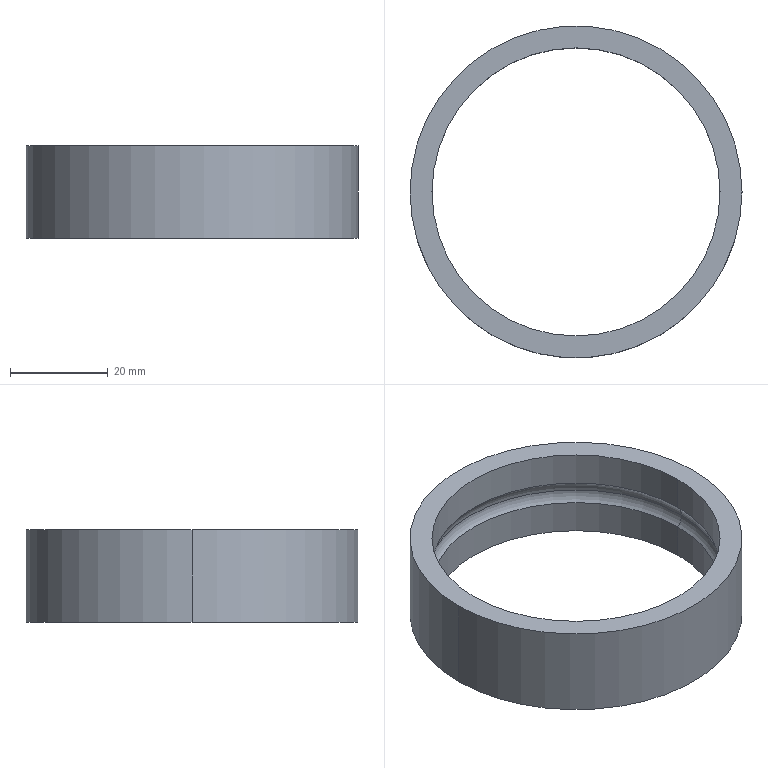Part | SolidWorks | 1 solid | 12 faces | box 68 x 68 x 19 mm | volume 16423 mm3 | cylinder 6 | torus 4 | plane 2 | commonest cylinder face diameters 59 x4 68 x2
STEP:
#1=CARTESIAN_POINT('',(-30.5,0.,-9.5));
#2=VERTEX_POINT('',#1);
#3=CARTESIAN_POINT('',(30.5,0.,-9.5));
#4=VERTEX_POINT('',#3);
#5=CARTESIAN_POINT('',(0.,0.,-9.5));
#6=DIRECTION('',(0.,0.,-1.));
#7=DIRECTION('',(-1.,0.,0.));
#8=AXIS2_PLACEMENT_3D('',#5,#6,#7);
#9=CIRCLE('',#8,30.5);
#10=EDGE_CURVE('',#2,#4,#9,.T.);
#11=ORIENTED_EDGE('',*,*,#10,.T.);
#12=CARTESIAN_POINT('',(29.5,0.,-7.051));
#13=VERTEX_POINT('',#12);
#14=CARTESIAN_POINT('',(27.,0.,-9.5));
#15=DIRECTION('',(0.,-1.,0.));
#16=DIRECTION('',(1.,0.,0.));
#17=AXIS2_PLACEMENT_3D('',#14,#15,#16);
#18=CIRCLE('',#17,3.5);
#19=EDGE_CURVE('',#4,#13,#18,.T.);
#20=ORIENTED_EDGE('',*,*,#19,.T.);
#21=CARTESIAN_POINT('',(-29.5,0.,-7.051));
#22=VERTEX_POINT('',#21);
#23=CARTESIAN_POINT('',(0.,0.,-7.051));
#24=DIRECTION('',(0.,0.,-1.));
#25=DIRECTION('',(-1.,0.,0.));
#26=AXIS2_PLACEMENT_3D('',#23,#24,#25);
#27=CIRCLE('',#26,29.5);
#28=EDGE_CURVE('',#22,#13,#27,.T.);
#29=ORIENTED_EDGE('',*,*,#28,.F.);
#30=CARTESIAN_POINT('',(-27.,0.,-9.5));
#31=DIRECTION('',(0.,1.,0.));
#32=DIRECTION('',(-1.,0.,0.));
#33=AXIS2_PLACEMENT_3D('',#30,#31,#32);
#34=CIRCLE('',#33,3.5);
#35=EDGE_CURVE('',#2,#22,#34,.T.);
#36=ORIENTED_EDGE('',*,*,#35,.F.);
#37=EDGE_LOOP('',(#11,#20,#29,#36));
#38=FACE_OUTER_BOUND('',#37,.T.);
#39=CARTESIAN_POINT('',(0.,0.,-9.5));
#40=DIRECTION('',(0.,0.,-1.));
#41=DIRECTION('',(1.,0.,0.));
#42=AXIS2_PLACEMENT_3D('',#39,#40,#41);
#43=TOROIDAL_SURFACE('',#42,27.,3.5);
#44=ADVANCED_FACE('',(#38),#43,.F.);
#45=CARTESIAN_POINT('',(29.5,0.,0.));
#46=VERTEX_POINT('',#45);
#47=CARTESIAN_POINT('',(29.5,0.,0.));
#48=DIRECTION('',(0.,0.,-1.));
#49=VECTOR('',#48,1000.);
#50=LINE('',#47,#49);
#51=EDGE_CURVE('',#46,#13,#50,.T.);
#52=ORIENTED_EDGE('',*,*,#51,.F.);
#53=CARTESIAN_POINT('',(-29.5,0.,0.));
#54=VERTEX_POINT('',#53);
#55=CARTESIAN_POINT('',(0.,0.,0.));
#56=DIRECTION('',(0.,0.,1.));
#57=DIRECTION('',(1.,0.,0.));
#58=AXIS2_PLACEMENT_3D('',#55,#56,#57);
#59=CIRCLE('',#58,29.5);
#60=EDGE_CURVE('',#46,#54,#59,.T.);
#61=ORIENTED_EDGE('',*,*,#60,.T.);
#62=CARTESIAN_POINT('',(-29.5,0.,0.));
#63=DIRECTION('',(0.,0.,-1.));
#64=VECTOR('',#63,1000.);
#65=LINE('',#62,#64);
#66=EDGE_CURVE('',#54,#22,#65,.T.);
#67=ORIENTED_EDGE('',*,*,#66,.T.);
#68=ORIENTED_EDGE('',*,*,#28,.T.);
#69=EDGE_LOOP('',(#52,#61,#67,#68));
#70=FACE_OUTER_BOUND('',#69,.T.);
#71=CARTESIAN_POINT('',(0.,0.,0.));
#72=DIRECTION('',(0.,0.,1.));
#73=DIRECTION('',(1.,0.,0.));
#74=AXIS2_PLACEMENT_3D('',#71,#72,#73);
#75=CYLINDRICAL_SURFACE('',#74,29.5);
#76=ADVANCED_FACE('',(#70),#75,.F.);
#77=CARTESIAN_POINT('',(0.,0.,0.));
#78=DIRECTION('',(0.,0.,1.));
#79=DIRECTION('',(-1.,0.,0.));
#80=AXIS2_PLACEMENT_3D('',#77,#78,#79);
#81=CIRCLE('',#80,29.5);
#82=EDGE_CURVE('',#54,#46,#81,.T.);
#83=ORIENTED_EDGE('',*,*,#82,.T.);
#84=ORIENTED_EDGE('',*,*,#51,.T.);
#85=CARTESIAN_POINT('',(0.,0.,-7.051));
#86=DIRECTION('',(0.,0.,-1.));
#87=DIRECTION('',(1.,0.,0.));
#88=AXIS2_PLACEMENT_3D('',#85,#86,#87);
#89=CIRCLE('',#88,29.5);
#90=EDGE_CURVE('',#13,#22,#89,.T.);
#91=ORIENTED_EDGE('',*,*,#90,.T.);
#92=ORIENTED_EDGE('',*,*,#66,.F.);
#93=EDGE_LOOP('',(#83,#84,#91,#92));
#94=FACE_OUTER_BOUND('',#93,.T.);
#95=CARTESIAN_POINT('',(0.,0.,0.));
#96=DIRECTION('',(0.,0.,1.));
#97=DIRECTION('',(1.,0.,0.));
#98=AXIS2_PLACEMENT_3D('',#95,#96,#97);
#99=CYLINDRICAL_SURFACE('',#98,29.5);
#100=ADVANCED_FACE('',(#94),#99,.F.);
#101=ORIENTED_EDGE('',*,*,#19,.F.);
#102=CARTESIAN_POINT('',(0.,0.,-9.5));
#103=DIRECTION('',(0.,0.,-1.));
#104=DIRECTION('',(1.,0.,0.));
#105=AXIS2_PLACEMENT_3D('',#102,#103,#104);
#106=CIRCLE('',#105,30.5);
#107=EDGE_CURVE('',#4,#2,#106,.T.);
#108=ORIENTED_EDGE('',*,*,#107,.T.);
#109=ORIENTED_EDGE('',*,*,#35,.T.);
#110=ORIENTED_EDGE('',*,*,#90,.F.);
#111=EDGE_LOOP('',(#101,#108,#109,#110));
#112=FACE_OUTER_BOUND('',#111,.T.);
#113=CARTESIAN_POINT('',(0.,0.,-9.5));
#114=DIRECTION('',(0.,0.,-1.));
#115=DIRECTION('',(-1.,0.,0.));
#116=AXIS2_PLACEMENT_3D('',#113,#114,#115);
#117=TOROIDAL_SURFACE('',#116,27.,3.5);
#118=ADVANCED_FACE('',(#112),#117,.F.);
#119=CARTESIAN_POINT('',(29.5,0.,-11.949));
#120=VERTEX_POINT('',#119);
#121=CARTESIAN_POINT('',(27.,0.,-9.5));
#122=DIRECTION('',(0.,-1.,0.));
#123=DIRECTION('',(0.7143,0.,-0.6999));
#124=AXIS2_PLACEMENT_3D('',#121,#122,#123);
#125=CIRCLE('',#124,3.5);
#126=EDGE_CURVE('',#120,#4,#125,.T.);
#127=ORIENTED_EDGE('',*,*,#126,.F.);
#128=CARTESIAN_POINT('',(-29.5,0.,-11.949));
#129=VERTEX_POINT('',#128);
#130=CARTESIAN_POINT('',(0.,0.,-11.949));
#131=DIRECTION('',(0.,0.,1.));
#132=DIRECTION('',(-1.,0.,0.));
#133=AXIS2_PLACEMENT_3D('',#130,#131,#132);
#134=CIRCLE('',#133,29.5);
#135=EDGE_CURVE('',#129,#120,#134,.T.);
#136=ORIENTED_EDGE('',*,*,#135,.F.);
#137=CARTESIAN_POINT('',(-27.,0.,-9.5));
#138=DIRECTION('',(0.,1.,0.));
#139=DIRECTION('',(-0.7143,0.,-0.6999));
#140=AXIS2_PLACEMENT_3D('',#137,#138,#139);
#141=CIRCLE('',#140,3.5);
#142=EDGE_CURVE('',#129,#2,#141,.T.);
#143=ORIENTED_EDGE('',*,*,#142,.T.);
#144=ORIENTED_EDGE('',*,*,#107,.F.);
#145=EDGE_LOOP('',(#127,#136,#143,#144));
#146=FACE_OUTER_BOUND('',#145,.T.);
#147=CARTESIAN_POINT('',(0.,0.,-9.5));
#148=DIRECTION('',(0.,0.,-1.));
#149=DIRECTION('',(-1.,0.,0.));
#150=AXIS2_PLACEMENT_3D('',#147,#148,#149);
#151=TOROIDAL_SURFACE('',#150,27.,3.5);
#152=ADVANCED_FACE('',(#146),#151,.F.);
#153=CARTESIAN_POINT('',(0.,0.,-11.949));
#154=DIRECTION('',(0.,0.,1.));
#155=DIRECTION('',(1.,0.,0.));
#156=AXIS2_PLACEMENT_3D('',#153,#154,#155);
#157=CIRCLE('',#156,29.5);
#158=EDGE_CURVE('',#120,#129,#157,.T.);
#159=ORIENTED_EDGE('',*,*,#158,.F.);
#160=ORIENTED_EDGE('',*,*,#126,.T.);
#161=ORIENTED_EDGE('',*,*,#10,.F.);
#162=ORIENTED_EDGE('',*,*,#142,.F.);
#163=EDGE_LOOP('',(#159,#160,#161,#162));
#164=FACE_OUTER_BOUND('',#163,.T.);
#165=CARTESIAN_POINT('',(0.,0.,-9.5));
#166=DIRECTION('',(0.,0.,-1.));
#167=DIRECTION('',(1.,0.,0.));
#168=AXIS2_PLACEMENT_3D('',#165,#166,#167);
#169=TOROIDAL_SURFACE('',#168,27.,3.5);
#170=ADVANCED_FACE('',(#164),#169,.F.);
#171=CARTESIAN_POINT('',(29.5,0.,-19.));
#172=VERTEX_POINT('',#171);
#173=CARTESIAN_POINT('',(29.5,0.,-11.949));
#174=DIRECTION('',(0.,0.,-1.));
#175=VECTOR('',#174,1000.);
#176=LINE('',#173,#175);
#177=EDGE_CURVE('',#120,#172,#176,.T.);
#178=ORIENTED_EDGE('',*,*,#177,.F.);
#179=ORIENTED_EDGE('',*,*,#158,.T.);
#180=CARTESIAN_POINT('',(-29.5,0.,-19.));
#181=VERTEX_POINT('',#180);
#182=CARTESIAN_POINT('',(-29.5,0.,-11.949));
#183=DIRECTION('',(0.,0.,-1.));
#184=VECTOR('',#183,1000.);
#185=LINE('',#182,#184);
#186=EDGE_CURVE('',#129,#181,#185,.T.);
#187=ORIENTED_EDGE('',*,*,#186,.T.);
#188=CARTESIAN_POINT('',(0.,0.,-19.));
#189=DIRECTION('',(0.,0.,-1.));
#190=DIRECTION('',(-1.,0.,0.));
#191=AXIS2_PLACEMENT_3D('',#188,#189,#190);
#192=CIRCLE('',#191,29.5);
#193=EDGE_CURVE('',#181,#172,#192,.T.);
#194=ORIENTED_EDGE('',*,*,#193,.T.);
#195=EDGE_LOOP('',(#178,#179,#187,#194));
#196=FACE_OUTER_BOUND('',#195,.T.);
#197=CARTESIAN_POINT('',(0.,0.,0.));
#198=DIRECTION('',(0.,0.,1.));
#199=DIRECTION('',(1.,0.,0.));
#200=AXIS2_PLACEMENT_3D('',#197,#198,#199);
#201=CYLINDRICAL_SURFACE('',#200,29.5);
#202=ADVANCED_FACE('',(#196),#201,.F.);
#203=ORIENTED_EDGE('',*,*,#135,.T.);
#204=ORIENTED_EDGE('',*,*,#177,.T.);
#205=CARTESIAN_POINT('',(0.,0.,-19.));
#206=DIRECTION('',(0.,0.,-1.));
#207=DIRECTION('',(1.,0.,0.));
#208=AXIS2_PLACEMENT_3D('',#205,#206,#207);
#209=CIRCLE('',#208,29.5);
#210=EDGE_CURVE('',#172,#181,#209,.T.);
#211=ORIENTED_EDGE('',*,*,#210,.T.);
#212=ORIENTED_EDGE('',*,*,#186,.F.);
#213=EDGE_LOOP('',(#203,#204,#211,#212));
#214=FACE_OUTER_BOUND('',#213,.T.);
#215=CARTESIAN_POINT('',(0.,0.,0.));
#216=DIRECTION('',(0.,0.,1.));
#217=DIRECTION('',(1.,0.,0.));
#218=AXIS2_PLACEMENT_3D('',#215,#216,#217);
#219=CYLINDRICAL_SURFACE('',#218,29.5);
#220=ADVANCED_FACE('',(#214),#219,.F.);
#221=ORIENTED_EDGE('',*,*,#193,.F.);
#222=ORIENTED_EDGE('',*,*,#210,.F.);
#223=EDGE_LOOP('',(#221,#222));
#224=FACE_BOUND('',#223,.T.);
#225=CARTESIAN_POINT('',(34.,0.,-19.));
#226=VERTEX_POINT('',#225);
#227=CARTESIAN_POINT('',(-34.,0.,-19.));
#228=VERTEX_POINT('',#227);
#229=CARTESIAN_POINT('',(0.,0.,-19.));
#230=DIRECTION('',(0.,0.,1.));
#231=DIRECTION('',(1.,0.,0.));
#232=AXIS2_PLACEMENT_3D('',#229,#230,#231);
#233=CIRCLE('',#232,34.);
#234=EDGE_CURVE('',#226,#228,#233,.T.);
#235=ORIENTED_EDGE('',*,*,#234,.F.);
#236=CARTESIAN_POINT('',(0.,0.,-19.));
#237=DIRECTION('',(0.,0.,1.));
#238=DIRECTION('',(-1.,0.,0.));
#239=AXIS2_PLACEMENT_3D('',#236,#237,#238);
#240=CIRCLE('',#239,34.);
#241=EDGE_CURVE('',#228,#226,#240,.T.);
#242=ORIENTED_EDGE('',*,*,#241,.F.);
#243=EDGE_LOOP('',(#235,#242));
#244=FACE_OUTER_BOUND('',#243,.T.);
#245=CARTESIAN_POINT('',(0.,-34.,-19.));
#246=DIRECTION('',(0.,0.,-1.));
#247=DIRECTION('',(0.,-1.,0.));
#248=AXIS2_PLACEMENT_3D('',#245,#246,#247);
#249=PLANE('',#248);
#250=ADVANCED_FACE('',(#224,#244),#249,.T.);
#251=CARTESIAN_POINT('',(34.,0.,0.));
#252=VERTEX_POINT('',#251);
#253=CARTESIAN_POINT('',(34.,0.,0.));
#254=DIRECTION('',(0.,0.,-1.));
#255=VECTOR('',#254,1000.);
#256=LINE('',#253,#255);
#257=EDGE_CURVE('',#252,#226,#256,.T.);
#258=ORIENTED_EDGE('',*,*,#257,.F.);
#259=CARTESIAN_POINT('',(-34.,0.,0.));
#260=VERTEX_POINT('',#259);
#261=CARTESIAN_POINT('',(0.,0.,0.));
#262=DIRECTION('',(0.,0.,-1.));
#263=DIRECTION('',(1.,0.,0.));
#264=AXIS2_PLACEMENT_3D('',#261,#262,#263);
#265=CIRCLE('',#264,34.);
#266=EDGE_CURVE('',#252,#260,#265,.T.);
#267=ORIENTED_EDGE('',*,*,#266,.T.);
#268=CARTESIAN_POINT('',(-34.,0.,0.));
#269=DIRECTION('',(0.,0.,-1.));
#270=VECTOR('',#269,1000.);
#271=LINE('',#268,#270);
#272=EDGE_CURVE('',#260,#228,#271,.T.);
#273=ORIENTED_EDGE('',*,*,#272,.T.);
#274=ORIENTED_EDGE('',*,*,#241,.T.);
#275=EDGE_LOOP('',(#258,#267,#273,#274));
#276=FACE_OUTER_BOUND('',#275,.T.);
#277=CARTESIAN_POINT('',(0.,0.,0.));
#278=DIRECTION('',(0.,0.,1.));
#279=DIRECTION('',(1.,0.,0.));
#280=AXIS2_PLACEMENT_3D('',#277,#278,#279);
#281=CYLINDRICAL_SURFACE('',#280,34.);
#282=ADVANCED_FACE('',(#276),#281,.T.);
#283=CARTESIAN_POINT('',(0.,0.,0.));
#284=DIRECTION('',(0.,0.,-1.));
#285=DIRECTION('',(-1.,0.,0.));
#286=AXIS2_PLACEMENT_3D('',#283,#284,#285);
#287=CIRCLE('',#286,34.);
#288=EDGE_CURVE('',#260,#252,#287,.T.);
#289=ORIENTED_EDGE('',*,*,#288,.T.);
#290=ORIENTED_EDGE('',*,*,#257,.T.);
#291=ORIENTED_EDGE('',*,*,#234,.T.);
#292=ORIENTED_EDGE('',*,*,#272,.F.);
#293=EDGE_LOOP('',(#289,#290,#291,#292));
#294=FACE_OUTER_BOUND('',#293,.T.);
#295=CARTESIAN_POINT('',(0.,0.,0.));
#296=DIRECTION('',(0.,0.,1.));
#297=DIRECTION('',(1.,0.,0.));
#298=AXIS2_PLACEMENT_3D('',#295,#296,#297);
#299=CYLINDRICAL_SURFACE('',#298,34.);
#300=ADVANCED_FACE('',(#294),#299,.T.);
#301=ORIENTED_EDGE('',*,*,#82,.F.);
#302=ORIENTED_EDGE('',*,*,#60,.F.);
#303=EDGE_LOOP('',(#301,#302));
#304=FACE_BOUND('',#303,.T.);
#305=ORIENTED_EDGE('',*,*,#266,.F.);
#306=ORIENTED_EDGE('',*,*,#288,.F.);
#307=EDGE_LOOP('',(#305,#306));
#308=FACE_OUTER_BOUND('',#307,.T.);
#309=CARTESIAN_POINT('',(0.,-29.5,0.));
#310=DIRECTION('',(0.,0.,1.));
#311=DIRECTION('',(1.,0.,0.));
#312=AXIS2_PLACEMENT_3D('',#309,#310,#311);
#313=PLANE('',#312);
#314=ADVANCED_FACE('',(#304,#308),#313,.T.);
#315=CLOSED_SHELL('',(#44,#76,#100,#118,#152,#170,#202,#220,#250,#282,#300,#314));
#316=MANIFOLD_SOLID_BREP('',#315);
#317=CARTESIAN_POINT('',(0.,0.,0.));
#318=DIRECTION('',(0.,0.,1.));
#319=DIRECTION('',(1.,0.,0.));
#320=AXIS2_PLACEMENT_3D('',#317,#318,#319);
#321=(LENGTH_UNIT()NAMED_UNIT(*)SI_UNIT(.MILLI.,.METRE.));
#322=UNCERTAINTY_MEASURE_WITH_UNIT(LENGTH_MEASURE(0.00001),#321,'','');
#323=(NAMED_UNIT(*)PLANE_ANGLE_UNIT()SI_UNIT($,.RADIAN.));
#324=(NAMED_UNIT(*)SI_UNIT($,.STERADIAN.)SOLID_ANGLE_UNIT());
#325=(GEOMETRIC_REPRESENTATION_CONTEXT(3)GLOBAL_UNCERTAINTY_ASSIGNED_CONTEXT((#322))GLOBAL_UNIT_ASSIGNED_CONTEXT((#321,#323,#324))REPRESENTATION_CONTEXT('',''));
#326=ADVANCED_BREP_SHAPE_REPRESENTATION('',(#316,#320),#325);